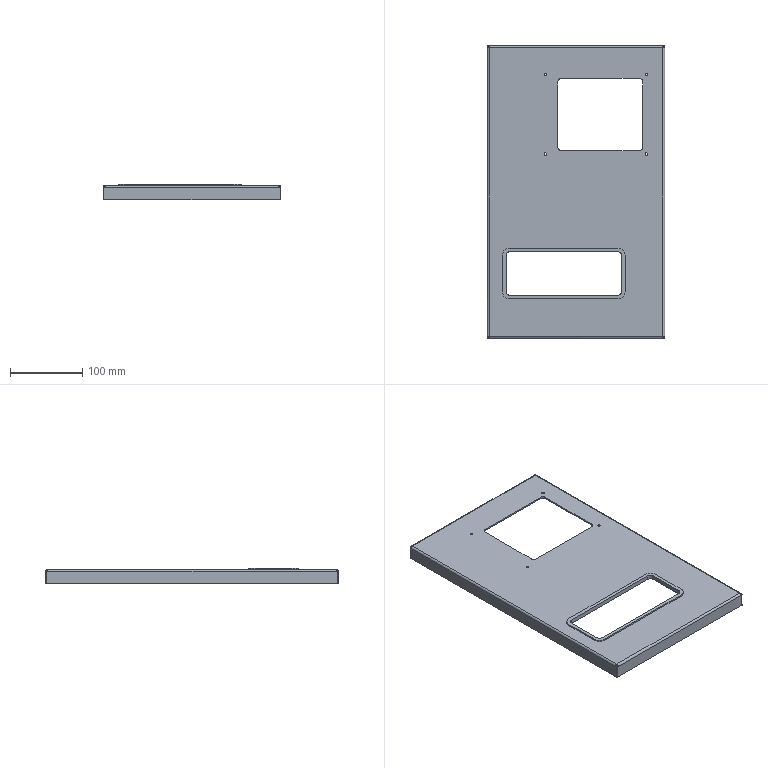Part | STEP file | Cabinet cover | 1 solid | 94 faces | box 246 x 406 x 22 mm | volume 265621 mm3 | plane 38 | cylinder 36 | spline 20 | commonest cylinder face diameters 3.3 x8 10 x8 20 x8 1.473 x4 2 x4 5.473 x4